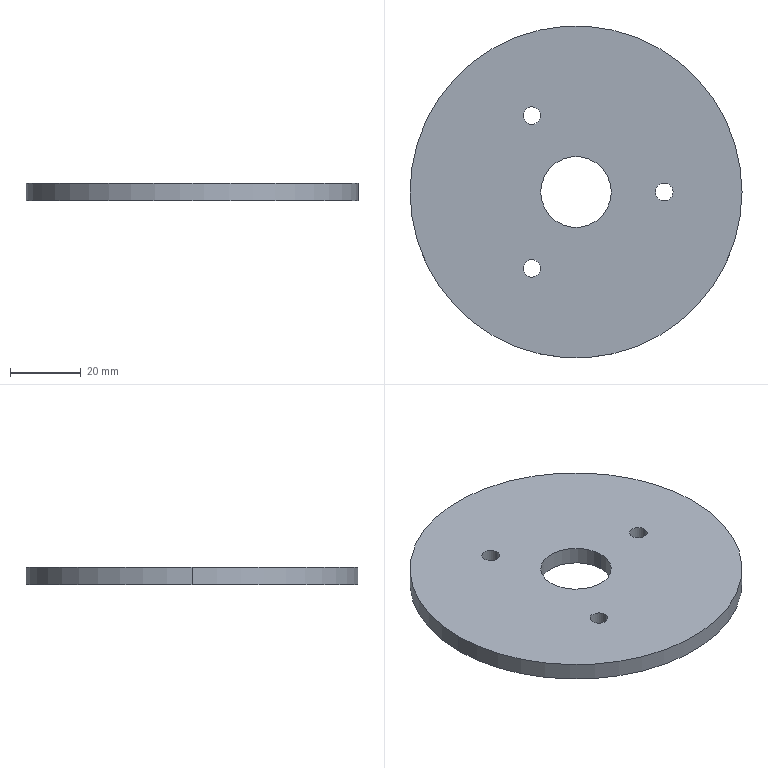Part | SolidWorks | features Extrusion 1 | 1 solid | 12 faces | box 94 x 94 x 5 mm | volume 32834 mm3 | cylinder 10 | plane 2 | commonest cylinder face diameters 5 x6 20 x2 94 x2
STEP:
#1=CARTESIAN_POINT('',(-15.,21.651,5.));
#2=VERTEX_POINT('',#1);
#3=CARTESIAN_POINT('',(-10.,21.651,5.));
#4=VERTEX_POINT('',#3);
#5=CARTESIAN_POINT('',(-12.5,21.651,5.));
#6=DIRECTION('',(0.,0.,1.));
#7=DIRECTION('',(1.,0.,0.));
#8=AXIS2_PLACEMENT_3D('',#5,#6,#7);
#9=CIRCLE('',#8,2.5);
#10=EDGE_CURVE('',#2,#4,#9,.T.);
#11=ORIENTED_EDGE('',*,*,#10,.T.);
#12=CARTESIAN_POINT('',(-10.,21.651,0.));
#13=VERTEX_POINT('',#12);
#14=CARTESIAN_POINT('',(-10.,21.651,5.));
#15=DIRECTION('',(0.,0.,-1.));
#16=VECTOR('',#15,1000.);
#17=LINE('',#14,#16);
#18=EDGE_CURVE('',#4,#13,#17,.T.);
#19=ORIENTED_EDGE('',*,*,#18,.T.);
#20=CARTESIAN_POINT('',(-15.,21.651,0.));
#21=VERTEX_POINT('',#20);
#22=CARTESIAN_POINT('',(-12.5,21.651,0.));
#23=DIRECTION('',(0.,0.,1.));
#24=DIRECTION('',(1.,0.,0.));
#25=AXIS2_PLACEMENT_3D('',#22,#23,#24);
#26=CIRCLE('',#25,2.5);
#27=EDGE_CURVE('',#21,#13,#26,.T.);
#28=ORIENTED_EDGE('',*,*,#27,.F.);
#29=CARTESIAN_POINT('',(-15.,21.651,5.));
#30=DIRECTION('',(0.,0.,-1.));
#31=VECTOR('',#30,1000.);
#32=LINE('',#29,#31);
#33=EDGE_CURVE('',#2,#21,#32,.T.);
#34=ORIENTED_EDGE('',*,*,#33,.F.);
#35=EDGE_LOOP('',(#11,#19,#28,#34));
#36=FACE_OUTER_BOUND('',#35,.T.);
#37=CARTESIAN_POINT('',(-12.5,21.651,5.));
#38=DIRECTION('',(0.,0.,-1.));
#39=DIRECTION('',(-1.,0.,0.));
#40=AXIS2_PLACEMENT_3D('',#37,#38,#39);
#41=CYLINDRICAL_SURFACE('',#40,2.5);
#42=ADVANCED_FACE('',(#36),#41,.F.);
#43=CARTESIAN_POINT('',(-15.,-21.651,5.));
#44=VERTEX_POINT('',#43);
#45=CARTESIAN_POINT('',(-10.,-21.651,5.));
#46=VERTEX_POINT('',#45);
#47=CARTESIAN_POINT('',(-12.5,-21.651,5.));
#48=DIRECTION('',(0.,0.,1.));
#49=DIRECTION('',(1.,0.,0.));
#50=AXIS2_PLACEMENT_3D('',#47,#48,#49);
#51=CIRCLE('',#50,2.5);
#52=EDGE_CURVE('',#44,#46,#51,.T.);
#53=ORIENTED_EDGE('',*,*,#52,.T.);
#54=CARTESIAN_POINT('',(-10.,-21.651,0.));
#55=VERTEX_POINT('',#54);
#56=CARTESIAN_POINT('',(-10.,-21.651,5.));
#57=DIRECTION('',(0.,0.,-1.));
#58=VECTOR('',#57,1000.);
#59=LINE('',#56,#58);
#60=EDGE_CURVE('',#46,#55,#59,.T.);
#61=ORIENTED_EDGE('',*,*,#60,.T.);
#62=CARTESIAN_POINT('',(-15.,-21.651,0.));
#63=VERTEX_POINT('',#62);
#64=CARTESIAN_POINT('',(-12.5,-21.651,0.));
#65=DIRECTION('',(0.,0.,1.));
#66=DIRECTION('',(1.,0.,0.));
#67=AXIS2_PLACEMENT_3D('',#64,#65,#66);
#68=CIRCLE('',#67,2.5);
#69=EDGE_CURVE('',#63,#55,#68,.T.);
#70=ORIENTED_EDGE('',*,*,#69,.F.);
#71=CARTESIAN_POINT('',(-15.,-21.651,5.));
#72=DIRECTION('',(0.,0.,-1.));
#73=VECTOR('',#72,1000.);
#74=LINE('',#71,#73);
#75=EDGE_CURVE('',#44,#63,#74,.T.);
#76=ORIENTED_EDGE('',*,*,#75,.F.);
#77=EDGE_LOOP('',(#53,#61,#70,#76));
#78=FACE_OUTER_BOUND('',#77,.T.);
#79=CARTESIAN_POINT('',(-12.5,-21.651,5.));
#80=DIRECTION('',(0.,0.,-1.));
#81=DIRECTION('',(-1.,0.,0.));
#82=AXIS2_PLACEMENT_3D('',#79,#80,#81);
#83=CYLINDRICAL_SURFACE('',#82,2.5);
#84=ADVANCED_FACE('',(#78),#83,.F.);
#85=CARTESIAN_POINT('',(22.5,0.,5.));
#86=VERTEX_POINT('',#85);
#87=CARTESIAN_POINT('',(27.5,0.,5.));
#88=VERTEX_POINT('',#87);
#89=CARTESIAN_POINT('',(25.,0.,5.));
#90=DIRECTION('',(0.,0.,1.));
#91=DIRECTION('',(1.,0.,0.));
#92=AXIS2_PLACEMENT_3D('',#89,#90,#91);
#93=CIRCLE('',#92,2.5);
#94=EDGE_CURVE('',#86,#88,#93,.T.);
#95=ORIENTED_EDGE('',*,*,#94,.T.);
#96=CARTESIAN_POINT('',(27.5,0.,0.));
#97=VERTEX_POINT('',#96);
#98=CARTESIAN_POINT('',(27.5,0.,5.));
#99=DIRECTION('',(0.,0.,-1.));
#100=VECTOR('',#99,1000.);
#101=LINE('',#98,#100);
#102=EDGE_CURVE('',#88,#97,#101,.T.);
#103=ORIENTED_EDGE('',*,*,#102,.T.);
#104=CARTESIAN_POINT('',(22.5,0.,0.));
#105=VERTEX_POINT('',#104);
#106=CARTESIAN_POINT('',(25.,0.,0.));
#107=DIRECTION('',(0.,0.,1.));
#108=DIRECTION('',(1.,0.,0.));
#109=AXIS2_PLACEMENT_3D('',#106,#107,#108);
#110=CIRCLE('',#109,2.5);
#111=EDGE_CURVE('',#105,#97,#110,.T.);
#112=ORIENTED_EDGE('',*,*,#111,.F.);
#113=CARTESIAN_POINT('',(22.5,0.,5.));
#114=DIRECTION('',(0.,0.,-1.));
#115=VECTOR('',#114,1000.);
#116=LINE('',#113,#115);
#117=EDGE_CURVE('',#86,#105,#116,.T.);
#118=ORIENTED_EDGE('',*,*,#117,.F.);
#119=EDGE_LOOP('',(#95,#103,#112,#118));
#120=FACE_OUTER_BOUND('',#119,.T.);
#121=CARTESIAN_POINT('',(25.,0.,5.));
#122=DIRECTION('',(0.,0.,-1.));
#123=DIRECTION('',(-1.,0.,0.));
#124=AXIS2_PLACEMENT_3D('',#121,#122,#123);
#125=CYLINDRICAL_SURFACE('',#124,2.5);
#126=ADVANCED_FACE('',(#120),#125,.F.);
#127=CARTESIAN_POINT('',(-10.,0.,5.));
#128=VERTEX_POINT('',#127);
#129=CARTESIAN_POINT('',(10.,0.,5.));
#130=VERTEX_POINT('',#129);
#131=CARTESIAN_POINT('',(0.,0.,5.));
#132=DIRECTION('',(0.,0.,1.));
#133=DIRECTION('',(1.,0.,0.));
#134=AXIS2_PLACEMENT_3D('',#131,#132,#133);
#135=CIRCLE('',#134,10.);
#136=EDGE_CURVE('',#128,#130,#135,.T.);
#137=ORIENTED_EDGE('',*,*,#136,.T.);
#138=CARTESIAN_POINT('',(10.,0.,0.));
#139=VERTEX_POINT('',#138);
#140=CARTESIAN_POINT('',(10.,0.,5.));
#141=DIRECTION('',(0.,0.,-1.));
#142=VECTOR('',#141,1000.);
#143=LINE('',#140,#142);
#144=EDGE_CURVE('',#130,#139,#143,.T.);
#145=ORIENTED_EDGE('',*,*,#144,.T.);
#146=CARTESIAN_POINT('',(-10.,0.,0.));
#147=VERTEX_POINT('',#146);
#148=CARTESIAN_POINT('',(0.,0.,0.));
#149=DIRECTION('',(0.,0.,1.));
#150=DIRECTION('',(1.,0.,0.));
#151=AXIS2_PLACEMENT_3D('',#148,#149,#150);
#152=CIRCLE('',#151,10.);
#153=EDGE_CURVE('',#147,#139,#152,.T.);
#154=ORIENTED_EDGE('',*,*,#153,.F.);
#155=CARTESIAN_POINT('',(-10.,0.,5.));
#156=DIRECTION('',(0.,0.,-1.));
#157=VECTOR('',#156,1000.);
#158=LINE('',#155,#157);
#159=EDGE_CURVE('',#128,#147,#158,.T.);
#160=ORIENTED_EDGE('',*,*,#159,.F.);
#161=EDGE_LOOP('',(#137,#145,#154,#160));
#162=FACE_OUTER_BOUND('',#161,.T.);
#163=CARTESIAN_POINT('',(0.,0.,5.));
#164=DIRECTION('',(0.,0.,-1.));
#165=DIRECTION('',(-1.,0.,0.));
#166=AXIS2_PLACEMENT_3D('',#163,#164,#165);
#167=CYLINDRICAL_SURFACE('',#166,10.);
#168=ADVANCED_FACE('',(#162),#167,.F.);
#169=CARTESIAN_POINT('',(47.,0.,5.));
#170=VERTEX_POINT('',#169);
#171=CARTESIAN_POINT('',(-47.,0.,5.));
#172=VERTEX_POINT('',#171);
#173=CARTESIAN_POINT('',(0.,0.,5.));
#174=DIRECTION('',(0.,0.,1.));
#175=DIRECTION('',(1.,0.,0.));
#176=AXIS2_PLACEMENT_3D('',#173,#174,#175);
#177=CIRCLE('',#176,47.);
#178=EDGE_CURVE('',#170,#172,#177,.T.);
#179=ORIENTED_EDGE('',*,*,#178,.F.);
#180=CARTESIAN_POINT('',(47.,0.,0.));
#181=VERTEX_POINT('',#180);
#182=CARTESIAN_POINT('',(47.,0.,5.));
#183=DIRECTION('',(0.,0.,-1.));
#184=VECTOR('',#183,1000.);
#185=LINE('',#182,#184);
#186=EDGE_CURVE('',#170,#181,#185,.T.);
#187=ORIENTED_EDGE('',*,*,#186,.T.);
#188=CARTESIAN_POINT('',(-47.,0.,0.));
#189=VERTEX_POINT('',#188);
#190=CARTESIAN_POINT('',(0.,0.,0.));
#191=DIRECTION('',(0.,0.,1.));
#192=DIRECTION('',(1.,0.,0.));
#193=AXIS2_PLACEMENT_3D('',#190,#191,#192);
#194=CIRCLE('',#193,47.);
#195=EDGE_CURVE('',#181,#189,#194,.T.);
#196=ORIENTED_EDGE('',*,*,#195,.T.);
#197=CARTESIAN_POINT('',(-47.,0.,5.));
#198=DIRECTION('',(0.,0.,-1.));
#199=VECTOR('',#198,1000.);
#200=LINE('',#197,#199);
#201=EDGE_CURVE('',#172,#189,#200,.T.);
#202=ORIENTED_EDGE('',*,*,#201,.F.);
#203=EDGE_LOOP('',(#179,#187,#196,#202));
#204=FACE_OUTER_BOUND('',#203,.T.);
#205=CARTESIAN_POINT('',(0.,0.,5.));
#206=DIRECTION('',(0.,0.,-1.));
#207=DIRECTION('',(-1.,0.,0.));
#208=AXIS2_PLACEMENT_3D('',#205,#206,#207);
#209=CYLINDRICAL_SURFACE('',#208,47.);
#210=ADVANCED_FACE('',(#204),#209,.T.);
#211=ORIENTED_EDGE('',*,*,#52,.F.);
#212=CARTESIAN_POINT('',(-12.5,-21.651,5.));
#213=DIRECTION('',(0.,0.,1.));
#214=DIRECTION('',(1.,0.,0.));
#215=AXIS2_PLACEMENT_3D('',#212,#213,#214);
#216=CIRCLE('',#215,2.5);
#217=EDGE_CURVE('',#46,#44,#216,.T.);
#218=ORIENTED_EDGE('',*,*,#217,.F.);
#219=EDGE_LOOP('',(#211,#218));
#220=FACE_BOUND('',#219,.T.);
#221=ORIENTED_EDGE('',*,*,#136,.F.);
#222=CARTESIAN_POINT('',(0.,0.,5.));
#223=DIRECTION('',(0.,0.,1.));
#224=DIRECTION('',(1.,0.,0.));
#225=AXIS2_PLACEMENT_3D('',#222,#223,#224);
#226=CIRCLE('',#225,10.);
#227=EDGE_CURVE('',#130,#128,#226,.T.);
#228=ORIENTED_EDGE('',*,*,#227,.F.);
#229=EDGE_LOOP('',(#221,#228));
#230=FACE_BOUND('',#229,.T.);
#231=CARTESIAN_POINT('',(0.,0.,5.));
#232=DIRECTION('',(0.,0.,1.));
#233=DIRECTION('',(1.,0.,0.));
#234=AXIS2_PLACEMENT_3D('',#231,#232,#233);
#235=CIRCLE('',#234,47.);
#236=EDGE_CURVE('',#172,#170,#235,.T.);
#237=ORIENTED_EDGE('',*,*,#236,.T.);
#238=ORIENTED_EDGE('',*,*,#178,.T.);
#239=EDGE_LOOP('',(#237,#238));
#240=FACE_OUTER_BOUND('',#239,.T.);
#241=ORIENTED_EDGE('',*,*,#94,.F.);
#242=CARTESIAN_POINT('',(25.,0.,5.));
#243=DIRECTION('',(0.,0.,1.));
#244=DIRECTION('',(1.,0.,0.));
#245=AXIS2_PLACEMENT_3D('',#242,#243,#244);
#246=CIRCLE('',#245,2.5);
#247=EDGE_CURVE('',#88,#86,#246,.T.);
#248=ORIENTED_EDGE('',*,*,#247,.F.);
#249=EDGE_LOOP('',(#241,#248));
#250=FACE_BOUND('',#249,.T.);
#251=ORIENTED_EDGE('',*,*,#10,.F.);
#252=CARTESIAN_POINT('',(-12.5,21.651,5.));
#253=DIRECTION('',(0.,0.,1.));
#254=DIRECTION('',(1.,0.,0.));
#255=AXIS2_PLACEMENT_3D('',#252,#253,#254);
#256=CIRCLE('',#255,2.5);
#257=EDGE_CURVE('',#4,#2,#256,.T.);
#258=ORIENTED_EDGE('',*,*,#257,.F.);
#259=EDGE_LOOP('',(#251,#258));
#260=FACE_BOUND('',#259,.T.);
#261=CARTESIAN_POINT('',(0.,0.,5.));
#262=DIRECTION('',(0.,0.,1.));
#263=DIRECTION('',(1.,0.,0.));
#264=AXIS2_PLACEMENT_3D('',#261,#262,#263);
#265=PLANE('',#264);
#266=ADVANCED_FACE('',(#220,#230,#240,#250,#260),#265,.T.);
#267=CARTESIAN_POINT('',(0.,0.,0.));
#268=DIRECTION('',(0.,0.,1.));
#269=DIRECTION('',(1.,0.,0.));
#270=AXIS2_PLACEMENT_3D('',#267,#268,#269);
#271=CIRCLE('',#270,47.);
#272=EDGE_CURVE('',#189,#181,#271,.T.);
#273=ORIENTED_EDGE('',*,*,#272,.F.);
#274=ORIENTED_EDGE('',*,*,#195,.F.);
#275=EDGE_LOOP('',(#273,#274));
#276=FACE_OUTER_BOUND('',#275,.T.);
#277=ORIENTED_EDGE('',*,*,#153,.T.);
#278=CARTESIAN_POINT('',(0.,0.,0.));
#279=DIRECTION('',(0.,0.,1.));
#280=DIRECTION('',(1.,0.,0.));
#281=AXIS2_PLACEMENT_3D('',#278,#279,#280);
#282=CIRCLE('',#281,10.);
#283=EDGE_CURVE('',#139,#147,#282,.T.);
#284=ORIENTED_EDGE('',*,*,#283,.T.);
#285=EDGE_LOOP('',(#277,#284));
#286=FACE_BOUND('',#285,.T.);
#287=ORIENTED_EDGE('',*,*,#111,.T.);
#288=CARTESIAN_POINT('',(25.,0.,0.));
#289=DIRECTION('',(0.,0.,1.));
#290=DIRECTION('',(1.,0.,0.));
#291=AXIS2_PLACEMENT_3D('',#288,#289,#290);
#292=CIRCLE('',#291,2.5);
#293=EDGE_CURVE('',#97,#105,#292,.T.);
#294=ORIENTED_EDGE('',*,*,#293,.T.);
#295=EDGE_LOOP('',(#287,#294));
#296=FACE_BOUND('',#295,.T.);
#297=ORIENTED_EDGE('',*,*,#69,.T.);
#298=CARTESIAN_POINT('',(-12.5,-21.651,0.));
#299=DIRECTION('',(0.,0.,1.));
#300=DIRECTION('',(1.,0.,0.));
#301=AXIS2_PLACEMENT_3D('',#298,#299,#300);
#302=CIRCLE('',#301,2.5);
#303=EDGE_CURVE('',#55,#63,#302,.T.);
#304=ORIENTED_EDGE('',*,*,#303,.T.);
#305=EDGE_LOOP('',(#297,#304));
#306=FACE_BOUND('',#305,.T.);
#307=ORIENTED_EDGE('',*,*,#27,.T.);
#308=CARTESIAN_POINT('',(-12.5,21.651,0.));
#309=DIRECTION('',(0.,0.,1.));
#310=DIRECTION('',(1.,0.,0.));
#311=AXIS2_PLACEMENT_3D('',#308,#309,#310);
#312=CIRCLE('',#311,2.5);
#313=EDGE_CURVE('',#13,#21,#312,.T.);
#314=ORIENTED_EDGE('',*,*,#313,.T.);
#315=EDGE_LOOP('',(#307,#314));
#316=FACE_BOUND('',#315,.T.);
#317=CARTESIAN_POINT('',(0.,0.,0.));
#318=DIRECTION('',(0.,0.,1.));
#319=DIRECTION('',(1.,0.,0.));
#320=AXIS2_PLACEMENT_3D('',#317,#318,#319);
#321=PLANE('',#320);
#322=ADVANCED_FACE('',(#276,#286,#296,#306,#316),#321,.F.);
#323=ORIENTED_EDGE('',*,*,#186,.F.);
#324=ORIENTED_EDGE('',*,*,#236,.F.);
#325=ORIENTED_EDGE('',*,*,#201,.T.);
#326=ORIENTED_EDGE('',*,*,#272,.T.);
#327=EDGE_LOOP('',(#323,#324,#325,#326));
#328=FACE_OUTER_BOUND('',#327,.T.);
#329=CARTESIAN_POINT('',(0.,0.,5.));
#330=DIRECTION('',(0.,0.,-1.));
#331=DIRECTION('',(-1.,0.,0.));
#332=AXIS2_PLACEMENT_3D('',#329,#330,#331);
#333=CYLINDRICAL_SURFACE('',#332,47.);
#334=ADVANCED_FACE('',(#328),#333,.T.);
#335=ORIENTED_EDGE('',*,*,#144,.F.);
#336=ORIENTED_EDGE('',*,*,#227,.T.);
#337=ORIENTED_EDGE('',*,*,#159,.T.);
#338=ORIENTED_EDGE('',*,*,#283,.F.);
#339=EDGE_LOOP('',(#335,#336,#337,#338));
#340=FACE_OUTER_BOUND('',#339,.T.);
#341=CARTESIAN_POINT('',(0.,0.,5.));
#342=DIRECTION('',(0.,0.,-1.));
#343=DIRECTION('',(-1.,0.,0.));
#344=AXIS2_PLACEMENT_3D('',#341,#342,#343);
#345=CYLINDRICAL_SURFACE('',#344,10.);
#346=ADVANCED_FACE('',(#340),#345,.F.);
#347=ORIENTED_EDGE('',*,*,#102,.F.);
#348=ORIENTED_EDGE('',*,*,#247,.T.);
#349=ORIENTED_EDGE('',*,*,#117,.T.);
#350=ORIENTED_EDGE('',*,*,#293,.F.);
#351=EDGE_LOOP('',(#347,#348,#349,#350));
#352=FACE_OUTER_BOUND('',#351,.T.);
#353=CARTESIAN_POINT('',(25.,0.,5.));
#354=DIRECTION('',(0.,0.,-1.));
#355=DIRECTION('',(-1.,0.,0.));
#356=AXIS2_PLACEMENT_3D('',#353,#354,#355);
#357=CYLINDRICAL_SURFACE('',#356,2.5);
#358=ADVANCED_FACE('',(#352),#357,.F.);
#359=ORIENTED_EDGE('',*,*,#60,.F.);
#360=ORIENTED_EDGE('',*,*,#217,.T.);
#361=ORIENTED_EDGE('',*,*,#75,.T.);
#362=ORIENTED_EDGE('',*,*,#303,.F.);
#363=EDGE_LOOP('',(#359,#360,#361,#362));
#364=FACE_OUTER_BOUND('',#363,.T.);
#365=CARTESIAN_POINT('',(-12.5,-21.651,5.));
#366=DIRECTION('',(0.,0.,-1.));
#367=DIRECTION('',(-1.,0.,0.));
#368=AXIS2_PLACEMENT_3D('',#365,#366,#367);
#369=CYLINDRICAL_SURFACE('',#368,2.5);
#370=ADVANCED_FACE('',(#364),#369,.F.);
#371=ORIENTED_EDGE('',*,*,#18,.F.);
#372=ORIENTED_EDGE('',*,*,#257,.T.);
#373=ORIENTED_EDGE('',*,*,#33,.T.);
#374=ORIENTED_EDGE('',*,*,#313,.F.);
#375=EDGE_LOOP('',(#371,#372,#373,#374));
#376=FACE_OUTER_BOUND('',#375,.T.);
#377=CARTESIAN_POINT('',(-12.5,21.651,5.));
#378=DIRECTION('',(0.,0.,-1.));
#379=DIRECTION('',(-1.,0.,0.));
#380=AXIS2_PLACEMENT_3D('',#377,#378,#379);
#381=CYLINDRICAL_SURFACE('',#380,2.5);
#382=ADVANCED_FACE('',(#376),#381,.F.);
#383=CLOSED_SHELL('',(#42,#84,#126,#168,#210,#266,#322,#334,#346,#358,#370,#382));
#384=MANIFOLD_SOLID_BREP('',#383);
#385=CARTESIAN_POINT('',(0.,0.,0.));
#386=DIRECTION('',(0.,0.,1.));
#387=DIRECTION('',(1.,0.,0.));
#388=AXIS2_PLACEMENT_3D('',#385,#386,#387);
#389=(LENGTH_UNIT()NAMED_UNIT(*)SI_UNIT(.MILLI.,.METRE.));
#390=UNCERTAINTY_MEASURE_WITH_UNIT(LENGTH_MEASURE(0.00001),#389,'','');
#391=(NAMED_UNIT(*)PLANE_ANGLE_UNIT()SI_UNIT($,.RADIAN.));
#392=(NAMED_UNIT(*)SI_UNIT($,.STERADIAN.)SOLID_ANGLE_UNIT());
#393=(GEOMETRIC_REPRESENTATION_CONTEXT(3)GLOBAL_UNCERTAINTY_ASSIGNED_CONTEXT((#390))GLOBAL_UNIT_ASSIGNED_CONTEXT((#389,#391,#392))REPRESENTATION_CONTEXT('',''));
#394=ADVANCED_BREP_SHAPE_REPRESENTATION('',(#384,#388),#393);